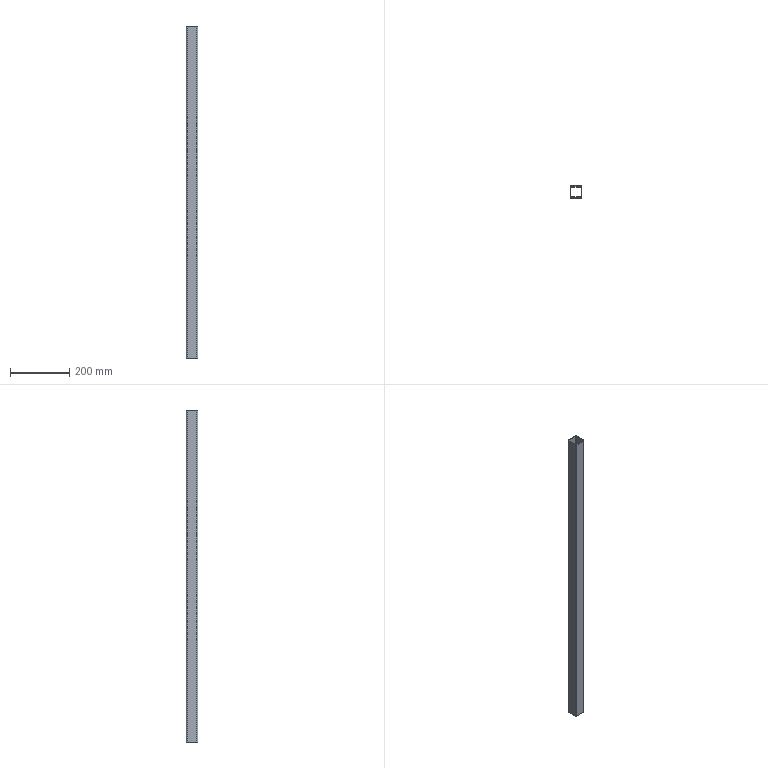Part | 1 solid | 14 faces | box 40 x 40 x 1120 mm | volume 477811 mm3 | plane 10 | cylinder 4 | commonest cylinder face diameters 9 x4
STEP:
#1=CARTESIAN_POINT('',(413.5,530.,-560.));
#2=VERTEX_POINT('',#1);
#3=CARTESIAN_POINT('',(418.,525.5,-560.));
#4=VERTEX_POINT('',#3);
#5=CARTESIAN_POINT('',(413.5,525.5,-560.));
#6=DIRECTION('',(0.,0.,-1.));
#7=DIRECTION('',(1.,0.,0.));
#8=AXIS2_PLACEMENT_3D('',#5,#6,#7);
#9=CIRCLE('',#8,4.5);
#10=EDGE_CURVE('',#2,#4,#9,.T.);
#11=ORIENTED_EDGE('',*,*,#10,.T.);
#12=CARTESIAN_POINT('',(418.,494.5,-560.));
#13=VERTEX_POINT('',#12);
#14=CARTESIAN_POINT('',(418.,40.,-560.));
#15=DIRECTION('',(0.,1.,0.));
#16=VECTOR('',#15,1000.);
#17=LINE('',#14,#16);
#18=EDGE_CURVE('',#13,#4,#17,.T.);
#19=ORIENTED_EDGE('',*,*,#18,.F.);
#20=CARTESIAN_POINT('',(413.5,490.,-560.));
#21=VERTEX_POINT('',#20);
#22=CARTESIAN_POINT('',(413.5,494.5,-560.));
#23=DIRECTION('',(0.,0.,-1.));
#24=DIRECTION('',(1.,0.,0.));
#25=AXIS2_PLACEMENT_3D('',#22,#23,#24);
#26=CIRCLE('',#25,4.5);
#27=EDGE_CURVE('',#13,#21,#26,.T.);
#28=ORIENTED_EDGE('',*,*,#27,.T.);
#29=CARTESIAN_POINT('',(382.5,490.,-560.));
#30=VERTEX_POINT('',#29);
#31=CARTESIAN_POINT('',(418.,490.,-560.));
#32=DIRECTION('',(1.,0.,0.));
#33=VECTOR('',#32,1000.);
#34=LINE('',#31,#33);
#35=EDGE_CURVE('',#30,#21,#34,.T.);
#36=ORIENTED_EDGE('',*,*,#35,.F.);
#37=CARTESIAN_POINT('',(378.,494.5,-560.));
#38=VERTEX_POINT('',#37);
#39=CARTESIAN_POINT('',(382.5,494.5,-560.));
#40=DIRECTION('',(0.,0.,-1.));
#41=DIRECTION('',(1.,0.,0.));
#42=AXIS2_PLACEMENT_3D('',#39,#40,#41);
#43=CIRCLE('',#42,4.5);
#44=EDGE_CURVE('',#30,#38,#43,.T.);
#45=ORIENTED_EDGE('',*,*,#44,.T.);
#46=CARTESIAN_POINT('',(378.,525.5,-560.));
#47=VERTEX_POINT('',#46);
#48=CARTESIAN_POINT('',(378.,40.,-560.));
#49=DIRECTION('',(0.,-1.,0.));
#50=VECTOR('',#49,1000.);
#51=LINE('',#48,#50);
#52=EDGE_CURVE('',#47,#38,#51,.T.);
#53=ORIENTED_EDGE('',*,*,#52,.F.);
#54=CARTESIAN_POINT('',(382.5,530.,-560.));
#55=VERTEX_POINT('',#54);
#56=CARTESIAN_POINT('',(382.5,525.5,-560.));
#57=DIRECTION('',(0.,0.,-1.));
#58=DIRECTION('',(1.,0.,0.));
#59=AXIS2_PLACEMENT_3D('',#56,#57,#58);
#60=CIRCLE('',#59,4.5);
#61=EDGE_CURVE('',#47,#55,#60,.T.);
#62=ORIENTED_EDGE('',*,*,#61,.T.);
#63=CARTESIAN_POINT('',(418.,530.,-560.));
#64=DIRECTION('',(1.,0.,0.));
#65=VECTOR('',#64,1000.);
#66=LINE('',#63,#65);
#67=EDGE_CURVE('',#55,#2,#66,.T.);
#68=ORIENTED_EDGE('',*,*,#67,.T.);
#69=EDGE_LOOP('',(#11,#19,#28,#36,#45,#53,#62,#68));
#70=FACE_OUTER_BOUND('',#69,.T.);
#71=CARTESIAN_POINT('',(415.,493.,-560.));
#72=VERTEX_POINT('',#71);
#73=CARTESIAN_POINT('',(381.,493.,-560.));
#74=VERTEX_POINT('',#73);
#75=CARTESIAN_POINT('',(418.,493.,-560.));
#76=DIRECTION('',(-1.,0.,0.));
#77=VECTOR('',#76,1000.);
#78=LINE('',#75,#77);
#79=EDGE_CURVE('',#72,#74,#78,.T.);
#80=ORIENTED_EDGE('',*,*,#79,.F.);
#81=CARTESIAN_POINT('',(415.,527.,-560.));
#82=VERTEX_POINT('',#81);
#83=CARTESIAN_POINT('',(415.,40.,-560.));
#84=DIRECTION('',(0.,-1.,0.));
#85=VECTOR('',#84,1000.);
#86=LINE('',#83,#85);
#87=EDGE_CURVE('',#82,#72,#86,.T.);
#88=ORIENTED_EDGE('',*,*,#87,.F.);
#89=CARTESIAN_POINT('',(381.,527.,-560.));
#90=VERTEX_POINT('',#89);
#91=CARTESIAN_POINT('',(418.,527.,-560.));
#92=DIRECTION('',(1.,0.,0.));
#93=VECTOR('',#92,1000.);
#94=LINE('',#91,#93);
#95=EDGE_CURVE('',#90,#82,#94,.T.);
#96=ORIENTED_EDGE('',*,*,#95,.F.);
#97=CARTESIAN_POINT('',(381.,40.,-560.));
#98=DIRECTION('',(0.,1.,0.));
#99=VECTOR('',#98,1000.);
#100=LINE('',#97,#99);
#101=EDGE_CURVE('',#74,#90,#100,.T.);
#102=ORIENTED_EDGE('',*,*,#101,.F.);
#103=EDGE_LOOP('',(#80,#88,#96,#102));
#104=FACE_BOUND('',#103,.T.);
#105=CARTESIAN_POINT('',(418.,40.,-560.));
#106=DIRECTION('',(0.,0.,1.));
#107=DIRECTION('',(1.,0.,0.));
#108=AXIS2_PLACEMENT_3D('',#105,#106,#107);
#109=PLANE('',#108);
#110=ADVANCED_FACE('',(#70,#104),#109,.F.);
#111=CARTESIAN_POINT('',(413.5,490.,560.));
#112=VERTEX_POINT('',#111);
#113=CARTESIAN_POINT('',(418.,494.5,560.));
#114=VERTEX_POINT('',#113);
#115=CARTESIAN_POINT('',(413.5,494.5,560.));
#116=DIRECTION('',(0.,0.,1.));
#117=DIRECTION('',(-1.,0.,0.));
#118=AXIS2_PLACEMENT_3D('',#115,#116,#117);
#119=CIRCLE('',#118,4.5);
#120=EDGE_CURVE('',#112,#114,#119,.T.);
#121=ORIENTED_EDGE('',*,*,#120,.T.);
#122=CARTESIAN_POINT('',(418.,525.5,560.));
#123=VERTEX_POINT('',#122);
#124=CARTESIAN_POINT('',(418.,40.,560.));
#125=DIRECTION('',(0.,-1.,0.));
#126=VECTOR('',#125,1000.);
#127=LINE('',#124,#126);
#128=EDGE_CURVE('',#123,#114,#127,.T.);
#129=ORIENTED_EDGE('',*,*,#128,.F.);
#130=CARTESIAN_POINT('',(413.5,530.,560.));
#131=VERTEX_POINT('',#130);
#132=CARTESIAN_POINT('',(413.5,525.5,560.));
#133=DIRECTION('',(0.,0.,1.));
#134=DIRECTION('',(-1.,0.,0.));
#135=AXIS2_PLACEMENT_3D('',#132,#133,#134);
#136=CIRCLE('',#135,4.5);
#137=EDGE_CURVE('',#123,#131,#136,.T.);
#138=ORIENTED_EDGE('',*,*,#137,.T.);
#139=CARTESIAN_POINT('',(382.5,530.,560.));
#140=VERTEX_POINT('',#139);
#141=CARTESIAN_POINT('',(418.,530.,560.));
#142=DIRECTION('',(-1.,0.,0.));
#143=VECTOR('',#142,1000.);
#144=LINE('',#141,#143);
#145=EDGE_CURVE('',#131,#140,#144,.T.);
#146=ORIENTED_EDGE('',*,*,#145,.T.);
#147=CARTESIAN_POINT('',(378.,525.5,560.));
#148=VERTEX_POINT('',#147);
#149=CARTESIAN_POINT('',(382.5,525.5,560.));
#150=DIRECTION('',(0.,0.,1.));
#151=DIRECTION('',(-1.,0.,0.));
#152=AXIS2_PLACEMENT_3D('',#149,#150,#151);
#153=CIRCLE('',#152,4.5);
#154=EDGE_CURVE('',#140,#148,#153,.T.);
#155=ORIENTED_EDGE('',*,*,#154,.T.);
#156=CARTESIAN_POINT('',(378.,494.5,560.));
#157=VERTEX_POINT('',#156);
#158=CARTESIAN_POINT('',(378.,23.5,560.));
#159=DIRECTION('',(0.,1.,0.));
#160=VECTOR('',#159,1000.);
#161=LINE('',#158,#160);
#162=EDGE_CURVE('',#157,#148,#161,.T.);
#163=ORIENTED_EDGE('',*,*,#162,.F.);
#164=CARTESIAN_POINT('',(382.5,490.,560.));
#165=VERTEX_POINT('',#164);
#166=CARTESIAN_POINT('',(382.5,494.5,560.));
#167=DIRECTION('',(0.,0.,1.));
#168=DIRECTION('',(-1.,0.,0.));
#169=AXIS2_PLACEMENT_3D('',#166,#167,#168);
#170=CIRCLE('',#169,4.5);
#171=EDGE_CURVE('',#157,#165,#170,.T.);
#172=ORIENTED_EDGE('',*,*,#171,.T.);
#173=CARTESIAN_POINT('',(378.,490.,560.));
#174=DIRECTION('',(-1.,0.,0.));
#175=VECTOR('',#174,1000.);
#176=LINE('',#173,#175);
#177=EDGE_CURVE('',#112,#165,#176,.T.);
#178=ORIENTED_EDGE('',*,*,#177,.F.);
#179=EDGE_LOOP('',(#121,#129,#138,#146,#155,#163,#172,#178));
#180=FACE_OUTER_BOUND('',#179,.T.);
#181=CARTESIAN_POINT('',(415.,527.,560.));
#182=VERTEX_POINT('',#181);
#183=CARTESIAN_POINT('',(381.,527.,560.));
#184=VERTEX_POINT('',#183);
#185=CARTESIAN_POINT('',(378.,527.,560.));
#186=DIRECTION('',(-1.,0.,0.));
#187=VECTOR('',#186,1000.);
#188=LINE('',#185,#187);
#189=EDGE_CURVE('',#182,#184,#188,.T.);
#190=ORIENTED_EDGE('',*,*,#189,.F.);
#191=CARTESIAN_POINT('',(415.,493.,560.));
#192=VERTEX_POINT('',#191);
#193=CARTESIAN_POINT('',(415.,40.,560.));
#194=DIRECTION('',(0.,1.,0.));
#195=VECTOR('',#194,1000.);
#196=LINE('',#193,#195);
#197=EDGE_CURVE('',#192,#182,#196,.T.);
#198=ORIENTED_EDGE('',*,*,#197,.F.);
#199=CARTESIAN_POINT('',(381.,493.,560.));
#200=VERTEX_POINT('',#199);
#201=CARTESIAN_POINT('',(378.,493.,560.));
#202=DIRECTION('',(1.,0.,0.));
#203=VECTOR('',#202,1000.);
#204=LINE('',#201,#203);
#205=EDGE_CURVE('',#200,#192,#204,.T.);
#206=ORIENTED_EDGE('',*,*,#205,.F.);
#207=CARTESIAN_POINT('',(381.,40.,560.));
#208=DIRECTION('',(0.,-1.,0.));
#209=VECTOR('',#208,1000.);
#210=LINE('',#207,#209);
#211=EDGE_CURVE('',#184,#200,#210,.T.);
#212=ORIENTED_EDGE('',*,*,#211,.F.);
#213=EDGE_LOOP('',(#190,#198,#206,#212));
#214=FACE_BOUND('',#213,.T.);
#215=CARTESIAN_POINT('',(378.,40.,560.));
#216=DIRECTION('',(0.,0.,-1.));
#217=DIRECTION('',(-1.,0.,0.));
#218=AXIS2_PLACEMENT_3D('',#215,#216,#217);
#219=PLANE('',#218);
#220=ADVANCED_FACE('',(#180,#214),#219,.F.);
#221=ORIENTED_EDGE('',*,*,#67,.F.);
#222=CARTESIAN_POINT('',(382.5,530.,560.));
#223=DIRECTION('',(0.,0.,1.));
#224=VECTOR('',#223,1000.);
#225=LINE('',#222,#224);
#226=EDGE_CURVE('',#55,#140,#225,.T.);
#227=ORIENTED_EDGE('',*,*,#226,.T.);
#228=ORIENTED_EDGE('',*,*,#145,.F.);
#229=CARTESIAN_POINT('',(413.5,530.,-410.));
#230=DIRECTION('',(0.,0.,-1.));
#231=VECTOR('',#230,1000.);
#232=LINE('',#229,#231);
#233=EDGE_CURVE('',#131,#2,#232,.T.);
#234=ORIENTED_EDGE('',*,*,#233,.T.);
#235=EDGE_LOOP('',(#221,#227,#228,#234));
#236=FACE_OUTER_BOUND('',#235,.T.);
#237=CARTESIAN_POINT('',(418.,530.,-410.));
#238=DIRECTION('',(0.,-1.,0.));
#239=DIRECTION('',(0.,0.,-1.));
#240=AXIS2_PLACEMENT_3D('',#237,#238,#239);
#241=PLANE('',#240);
#242=ADVANCED_FACE('',(#236),#241,.F.);
#243=ORIENTED_EDGE('',*,*,#162,.T.);
#244=CARTESIAN_POINT('',(378.,525.5,-560.));
#245=DIRECTION('',(0.,0.,-1.));
#246=VECTOR('',#245,1000.);
#247=LINE('',#244,#246);
#248=EDGE_CURVE('',#148,#47,#247,.T.);
#249=ORIENTED_EDGE('',*,*,#248,.T.);
#250=ORIENTED_EDGE('',*,*,#52,.T.);
#251=CARTESIAN_POINT('',(378.,494.5,560.));
#252=DIRECTION('',(0.,0.,1.));
#253=VECTOR('',#252,1000.);
#254=LINE('',#251,#253);
#255=EDGE_CURVE('',#38,#157,#254,.T.);
#256=ORIENTED_EDGE('',*,*,#255,.T.);
#257=EDGE_LOOP('',(#243,#249,#250,#256));
#258=FACE_OUTER_BOUND('',#257,.T.);
#259=CARTESIAN_POINT('',(378.,23.5,-410.));
#260=DIRECTION('',(-1.,0.,0.));
#261=DIRECTION('',(0.,0.,1.));
#262=AXIS2_PLACEMENT_3D('',#259,#260,#261);
#263=PLANE('',#262);
#264=ADVANCED_FACE('',(#258),#263,.T.);
#265=ORIENTED_EDGE('',*,*,#18,.T.);
#266=CARTESIAN_POINT('',(418.,525.5,-590.));
#267=DIRECTION('',(0.,0.,1.));
#268=VECTOR('',#267,1000.);
#269=LINE('',#266,#268);
#270=EDGE_CURVE('',#4,#123,#269,.T.);
#271=ORIENTED_EDGE('',*,*,#270,.T.);
#272=ORIENTED_EDGE('',*,*,#128,.T.);
#273=CARTESIAN_POINT('',(418.,494.5,-590.));
#274=DIRECTION('',(0.,0.,-1.));
#275=VECTOR('',#274,1000.);
#276=LINE('',#273,#275);
#277=EDGE_CURVE('',#114,#13,#276,.T.);
#278=ORIENTED_EDGE('',*,*,#277,.T.);
#279=EDGE_LOOP('',(#265,#271,#272,#278));
#280=FACE_OUTER_BOUND('',#279,.T.);
#281=CARTESIAN_POINT('',(418.,530.,-590.));
#282=DIRECTION('',(-1.,0.,0.));
#283=DIRECTION('',(0.,0.,1.));
#284=AXIS2_PLACEMENT_3D('',#281,#282,#283);
#285=PLANE('',#284);
#286=ADVANCED_FACE('',(#280),#285,.F.);
#287=ORIENTED_EDGE('',*,*,#35,.T.);
#288=CARTESIAN_POINT('',(413.5,490.,-560.002));
#289=DIRECTION('',(0.,0.,1.));
#290=VECTOR('',#289,1000.);
#291=LINE('',#288,#290);
#292=EDGE_CURVE('',#21,#112,#291,.T.);
#293=ORIENTED_EDGE('',*,*,#292,.T.);
#294=ORIENTED_EDGE('',*,*,#177,.T.);
#295=CARTESIAN_POINT('',(382.5,490.,-560.));
#296=DIRECTION('',(0.,0.,-1.));
#297=VECTOR('',#296,1000.);
#298=LINE('',#295,#297);
#299=EDGE_CURVE('',#165,#30,#298,.T.);
#300=ORIENTED_EDGE('',*,*,#299,.T.);
#301=EDGE_LOOP('',(#287,#293,#294,#300));
#302=FACE_OUTER_BOUND('',#301,.T.);
#303=CARTESIAN_POINT('',(418.,490.,-560.002));
#304=DIRECTION('',(0.,1.,0.));
#305=DIRECTION('',(0.,0.,1.));
#306=AXIS2_PLACEMENT_3D('',#303,#304,#305);
#307=PLANE('',#306);
#308=ADVANCED_FACE('',(#302),#307,.F.);
#309=CARTESIAN_POINT('',(415.,527.,-480.));
#310=DIRECTION('',(0.,0.,1.));
#311=VECTOR('',#310,1000.);
#312=LINE('',#309,#311);
#313=EDGE_CURVE('',#82,#182,#312,.T.);
#314=ORIENTED_EDGE('',*,*,#313,.T.);
#315=ORIENTED_EDGE('',*,*,#189,.T.);
#316=CARTESIAN_POINT('',(381.,527.,-410.));
#317=DIRECTION('',(0.,0.,-1.));
#318=VECTOR('',#317,1000.);
#319=LINE('',#316,#318);
#320=EDGE_CURVE('',#184,#90,#319,.T.);
#321=ORIENTED_EDGE('',*,*,#320,.T.);
#322=ORIENTED_EDGE('',*,*,#95,.T.);
#323=EDGE_LOOP('',(#314,#315,#321,#322));
#324=FACE_OUTER_BOUND('',#323,.T.);
#325=CARTESIAN_POINT('',(-142.,527.,-520.));
#326=DIRECTION('',(0.,-1.,0.));
#327=DIRECTION('',(0.,0.,-1.));
#328=AXIS2_PLACEMENT_3D('',#325,#326,#327);
#329=PLANE('',#328);
#330=ADVANCED_FACE('',(#324),#329,.T.);
#331=ORIENTED_EDGE('',*,*,#101,.T.);
#332=ORIENTED_EDGE('',*,*,#320,.F.);
#333=ORIENTED_EDGE('',*,*,#211,.T.);
#334=CARTESIAN_POINT('',(381.,493.,-450.002));
#335=DIRECTION('',(0.,0.,-1.));
#336=VECTOR('',#335,1000.);
#337=LINE('',#334,#336);
#338=EDGE_CURVE('',#200,#74,#337,.T.);
#339=ORIENTED_EDGE('',*,*,#338,.T.);
#340=EDGE_LOOP('',(#331,#332,#333,#339));
#341=FACE_OUTER_BOUND('',#340,.T.);
#342=CARTESIAN_POINT('',(381.,850.,-410.));
#343=DIRECTION('',(1.,0.,0.));
#344=DIRECTION('',(0.,0.,-1.));
#345=AXIS2_PLACEMENT_3D('',#342,#343,#344);
#346=PLANE('',#345);
#347=ADVANCED_FACE('',(#341),#346,.T.);
#348=ORIENTED_EDGE('',*,*,#79,.T.);
#349=ORIENTED_EDGE('',*,*,#338,.F.);
#350=ORIENTED_EDGE('',*,*,#205,.T.);
#351=CARTESIAN_POINT('',(415.,493.,-480.));
#352=DIRECTION('',(0.,0.,-1.));
#353=VECTOR('',#352,1000.);
#354=LINE('',#351,#353);
#355=EDGE_CURVE('',#192,#72,#354,.T.);
#356=ORIENTED_EDGE('',*,*,#355,.T.);
#357=EDGE_LOOP('',(#348,#349,#350,#356));
#358=FACE_OUTER_BOUND('',#357,.T.);
#359=CARTESIAN_POINT('',(418.,493.,-450.002));
#360=DIRECTION('',(0.,1.,0.));
#361=DIRECTION('',(0.,0.,1.));
#362=AXIS2_PLACEMENT_3D('',#359,#360,#361);
#363=PLANE('',#362);
#364=ADVANCED_FACE('',(#358),#363,.T.);
#365=ORIENTED_EDGE('',*,*,#87,.T.);
#366=ORIENTED_EDGE('',*,*,#355,.F.);
#367=ORIENTED_EDGE('',*,*,#197,.T.);
#368=ORIENTED_EDGE('',*,*,#313,.F.);
#369=EDGE_LOOP('',(#365,#366,#367,#368));
#370=FACE_OUTER_BOUND('',#369,.T.);
#371=CARTESIAN_POINT('',(415.,530.,-480.));
#372=DIRECTION('',(-1.,0.,0.));
#373=DIRECTION('',(0.,0.,1.));
#374=AXIS2_PLACEMENT_3D('',#371,#372,#373);
#375=PLANE('',#374);
#376=ADVANCED_FACE('',(#370),#375,.T.);
#377=ORIENTED_EDGE('',*,*,#154,.F.);
#378=ORIENTED_EDGE('',*,*,#226,.F.);
#379=ORIENTED_EDGE('',*,*,#61,.F.);
#380=ORIENTED_EDGE('',*,*,#248,.F.);
#381=EDGE_LOOP('',(#377,#378,#379,#380));
#382=FACE_OUTER_BOUND('',#381,.T.);
#383=CARTESIAN_POINT('',(382.5,525.5,-410.));
#384=DIRECTION('',(0.,0.,1.));
#385=DIRECTION('',(1.,0.,0.));
#386=AXIS2_PLACEMENT_3D('',#383,#384,#385);
#387=CYLINDRICAL_SURFACE('',#386,4.5);
#388=ADVANCED_FACE('',(#382),#387,.T.);
#389=ORIENTED_EDGE('',*,*,#10,.F.);
#390=ORIENTED_EDGE('',*,*,#233,.F.);
#391=ORIENTED_EDGE('',*,*,#137,.F.);
#392=ORIENTED_EDGE('',*,*,#270,.F.);
#393=EDGE_LOOP('',(#389,#390,#391,#392));
#394=FACE_OUTER_BOUND('',#393,.T.);
#395=CARTESIAN_POINT('',(413.5,525.5,-590.));
#396=DIRECTION('',(0.,0.,1.));
#397=DIRECTION('',(1.,0.,0.));
#398=AXIS2_PLACEMENT_3D('',#395,#396,#397);
#399=CYLINDRICAL_SURFACE('',#398,4.5);
#400=ADVANCED_FACE('',(#394),#399,.T.);
#401=ORIENTED_EDGE('',*,*,#27,.F.);
#402=ORIENTED_EDGE('',*,*,#277,.F.);
#403=ORIENTED_EDGE('',*,*,#120,.F.);
#404=ORIENTED_EDGE('',*,*,#292,.F.);
#405=EDGE_LOOP('',(#401,#402,#403,#404));
#406=FACE_OUTER_BOUND('',#405,.T.);
#407=CARTESIAN_POINT('',(413.5,494.5,-560.002));
#408=DIRECTION('',(0.,0.,1.));
#409=DIRECTION('',(1.,0.,0.));
#410=AXIS2_PLACEMENT_3D('',#407,#408,#409);
#411=CYLINDRICAL_SURFACE('',#410,4.5);
#412=ADVANCED_FACE('',(#406),#411,.T.);
#413=ORIENTED_EDGE('',*,*,#44,.F.);
#414=ORIENTED_EDGE('',*,*,#299,.F.);
#415=ORIENTED_EDGE('',*,*,#171,.F.);
#416=ORIENTED_EDGE('',*,*,#255,.F.);
#417=EDGE_LOOP('',(#413,#414,#415,#416));
#418=FACE_OUTER_BOUND('',#417,.T.);
#419=CARTESIAN_POINT('',(382.5,494.5,-410.));
#420=DIRECTION('',(0.,0.,-1.));
#421=DIRECTION('',(-1.,0.,0.));
#422=AXIS2_PLACEMENT_3D('',#419,#420,#421);
#423=CYLINDRICAL_SURFACE('',#422,4.5);
#424=ADVANCED_FACE('',(#418),#423,.T.);
#425=CLOSED_SHELL('',(#110,#220,#242,#264,#286,#308,#330,#347,#364,#376,#388,#400,#412,#424));
#426=MANIFOLD_SOLID_BREP('',#425);
#427=CARTESIAN_POINT('',(0.,0.,0.));
#428=DIRECTION('',(0.,0.,1.));
#429=DIRECTION('',(1.,0.,0.));
#430=AXIS2_PLACEMENT_3D('',#427,#428,#429);
#431=(LENGTH_UNIT()NAMED_UNIT(*)SI_UNIT(.MILLI.,.METRE.));
#432=UNCERTAINTY_MEASURE_WITH_UNIT(LENGTH_MEASURE(0.00001),#431,'','');
#433=(NAMED_UNIT(*)PLANE_ANGLE_UNIT()SI_UNIT($,.RADIAN.));
#434=(NAMED_UNIT(*)SI_UNIT($,.STERADIAN.)SOLID_ANGLE_UNIT());
#435=(GEOMETRIC_REPRESENTATION_CONTEXT(3)GLOBAL_UNCERTAINTY_ASSIGNED_CONTEXT((#432))GLOBAL_UNIT_ASSIGNED_CONTEXT((#431,#433,#434))REPRESENTATION_CONTEXT('',''));
#436=ADVANCED_BREP_SHAPE_REPRESENTATION('',(#426,#430),#435);